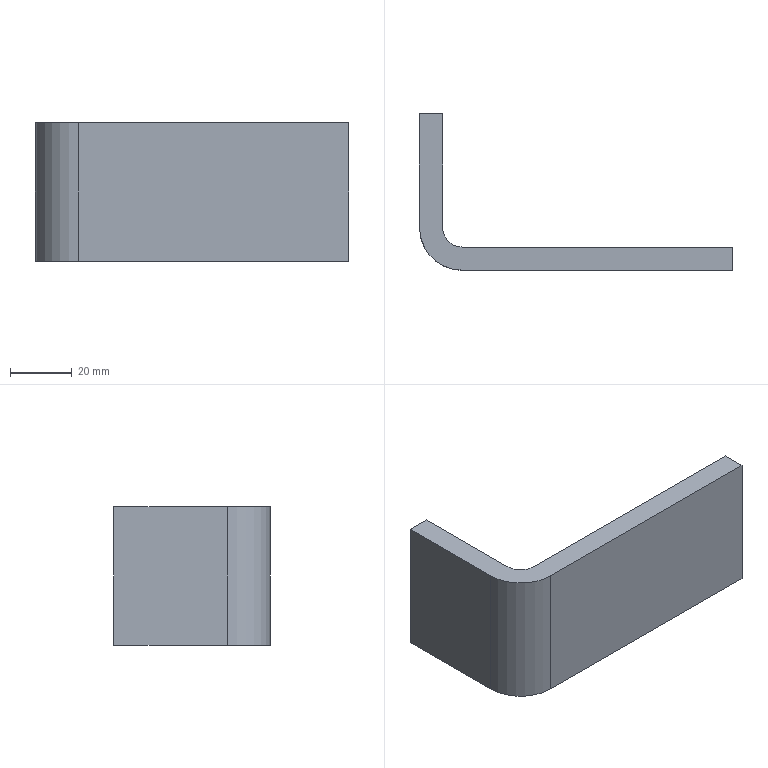Part | SolidWorks | features Extrusion 1 | 1 solid | 10 faces | box 101.6 x 50.8 x 45 mm | volume 47441 mm3 | plane 8 | cylinder 2 | commonest cylinder face diameters 12.7 x1 27.7 x1
STEP:
#1=CARTESIAN_POINT('',(-16.453,5.356,0.));
#2=VERTEX_POINT('',#1);
#3=CARTESIAN_POINT('',(-23.953,5.356,0.));
#4=VERTEX_POINT('',#3);
#5=CARTESIAN_POINT('',(-16.453,5.356,0.));
#6=DIRECTION('',(-1.,0.,0.));
#7=VECTOR('',#6,1000.);
#8=LINE('',#5,#7);
#9=EDGE_CURVE('',#2,#4,#8,.T.);
#10=ORIENTED_EDGE('',*,*,#9,.T.);
#11=CARTESIAN_POINT('',(-23.953,5.356,45.));
#12=VERTEX_POINT('',#11);
#13=CARTESIAN_POINT('',(-23.953,5.356,45.));
#14=DIRECTION('',(0.,0.,-1.));
#15=VECTOR('',#14,1000.);
#16=LINE('',#13,#15);
#17=EDGE_CURVE('',#12,#4,#16,.T.);
#18=ORIENTED_EDGE('',*,*,#17,.F.);
#19=CARTESIAN_POINT('',(-16.453,5.356,45.));
#20=VERTEX_POINT('',#19);
#21=CARTESIAN_POINT('',(-16.453,5.356,45.));
#22=DIRECTION('',(-1.,0.,0.));
#23=VECTOR('',#22,1000.);
#24=LINE('',#21,#23);
#25=EDGE_CURVE('',#20,#12,#24,.T.);
#26=ORIENTED_EDGE('',*,*,#25,.F.);
#27=CARTESIAN_POINT('',(-16.453,5.356,45.));
#28=DIRECTION('',(0.,0.,-1.));
#29=VECTOR('',#28,1000.);
#30=LINE('',#27,#29);
#31=EDGE_CURVE('',#20,#2,#30,.T.);
#32=ORIENTED_EDGE('',*,*,#31,.T.);
#33=EDGE_LOOP('',(#10,#18,#26,#32));
#34=FACE_OUTER_BOUND('',#33,.T.);
#35=CARTESIAN_POINT('',(-16.453,5.356,45.));
#36=DIRECTION('',(0.,-1.,0.));
#37=DIRECTION('',(1.,0.,0.));
#38=AXIS2_PLACEMENT_3D('',#35,#36,#37);
#39=PLANE('',#38);
#40=ADVANCED_FACE('',(#34),#39,.F.);
#41=CARTESIAN_POINT('',(-23.953,-31.594,0.));
#42=VERTEX_POINT('',#41);
#43=CARTESIAN_POINT('',(-23.953,5.356,0.));
#44=DIRECTION('',(0.,-1.,0.));
#45=VECTOR('',#44,1000.);
#46=LINE('',#43,#45);
#47=EDGE_CURVE('',#4,#42,#46,.T.);
#48=ORIENTED_EDGE('',*,*,#47,.T.);
#49=CARTESIAN_POINT('',(-23.953,-31.594,45.));
#50=VERTEX_POINT('',#49);
#51=CARTESIAN_POINT('',(-23.953,-31.594,45.));
#52=DIRECTION('',(0.,0.,-1.));
#53=VECTOR('',#52,1000.);
#54=LINE('',#51,#53);
#55=EDGE_CURVE('',#50,#42,#54,.T.);
#56=ORIENTED_EDGE('',*,*,#55,.F.);
#57=CARTESIAN_POINT('',(-23.953,5.356,45.));
#58=DIRECTION('',(0.,-1.,0.));
#59=VECTOR('',#58,1000.);
#60=LINE('',#57,#59);
#61=EDGE_CURVE('',#12,#50,#60,.T.);
#62=ORIENTED_EDGE('',*,*,#61,.F.);
#63=ORIENTED_EDGE('',*,*,#17,.T.);
#64=EDGE_LOOP('',(#48,#56,#62,#63));
#65=FACE_OUTER_BOUND('',#64,.T.);
#66=CARTESIAN_POINT('',(-23.953,5.356,45.));
#67=DIRECTION('',(1.,0.,0.));
#68=DIRECTION('',(0.,1.,0.));
#69=AXIS2_PLACEMENT_3D('',#66,#67,#68);
#70=PLANE('',#69);
#71=ADVANCED_FACE('',(#65),#70,.F.);
#72=CARTESIAN_POINT('',(-10.103,-45.444,0.));
#73=VERTEX_POINT('',#72);
#74=CARTESIAN_POINT('',(-10.103,-31.594,0.));
#75=DIRECTION('',(0.,0.,1.));
#76=DIRECTION('',(1.,0.,0.));
#77=AXIS2_PLACEMENT_3D('',#74,#75,#76);
#78=CIRCLE('',#77,13.85);
#79=EDGE_CURVE('',#42,#73,#78,.T.);
#80=ORIENTED_EDGE('',*,*,#79,.T.);
#81=CARTESIAN_POINT('',(-10.103,-45.444,45.));
#82=VERTEX_POINT('',#81);
#83=CARTESIAN_POINT('',(-10.103,-45.444,45.));
#84=DIRECTION('',(0.,0.,-1.));
#85=VECTOR('',#84,1000.);
#86=LINE('',#83,#85);
#87=EDGE_CURVE('',#82,#73,#86,.T.);
#88=ORIENTED_EDGE('',*,*,#87,.F.);
#89=CARTESIAN_POINT('',(-10.103,-31.594,45.));
#90=DIRECTION('',(0.,0.,1.));
#91=DIRECTION('',(1.,0.,0.));
#92=AXIS2_PLACEMENT_3D('',#89,#90,#91);
#93=CIRCLE('',#92,13.85);
#94=EDGE_CURVE('',#50,#82,#93,.T.);
#95=ORIENTED_EDGE('',*,*,#94,.F.);
#96=ORIENTED_EDGE('',*,*,#55,.T.);
#97=EDGE_LOOP('',(#80,#88,#95,#96));
#98=FACE_OUTER_BOUND('',#97,.T.);
#99=CARTESIAN_POINT('',(-10.103,-31.594,45.));
#100=DIRECTION('',(0.,0.,-1.));
#101=DIRECTION('',(-1.,0.,0.));
#102=AXIS2_PLACEMENT_3D('',#99,#100,#101);
#103=CYLINDRICAL_SURFACE('',#102,13.85);
#104=ADVANCED_FACE('',(#98),#103,.T.);
#105=CARTESIAN_POINT('',(77.647,-45.444,0.));
#106=VERTEX_POINT('',#105);
#107=CARTESIAN_POINT('',(-10.103,-45.444,0.));
#108=DIRECTION('',(1.,0.,0.));
#109=VECTOR('',#108,1000.);
#110=LINE('',#107,#109);
#111=EDGE_CURVE('',#73,#106,#110,.T.);
#112=ORIENTED_EDGE('',*,*,#111,.T.);
#113=CARTESIAN_POINT('',(77.647,-45.444,45.));
#114=VERTEX_POINT('',#113);
#115=CARTESIAN_POINT('',(77.647,-45.444,45.));
#116=DIRECTION('',(0.,0.,-1.));
#117=VECTOR('',#116,1000.);
#118=LINE('',#115,#117);
#119=EDGE_CURVE('',#114,#106,#118,.T.);
#120=ORIENTED_EDGE('',*,*,#119,.F.);
#121=CARTESIAN_POINT('',(-10.103,-45.444,45.));
#122=DIRECTION('',(1.,0.,0.));
#123=VECTOR('',#122,1000.);
#124=LINE('',#121,#123);
#125=EDGE_CURVE('',#82,#114,#124,.T.);
#126=ORIENTED_EDGE('',*,*,#125,.F.);
#127=ORIENTED_EDGE('',*,*,#87,.T.);
#128=EDGE_LOOP('',(#112,#120,#126,#127));
#129=FACE_OUTER_BOUND('',#128,.T.);
#130=CARTESIAN_POINT('',(-10.103,-45.444,45.));
#131=DIRECTION('',(0.,1.,0.));
#132=DIRECTION('',(0.,0.,1.));
#133=AXIS2_PLACEMENT_3D('',#130,#131,#132);
#134=PLANE('',#133);
#135=ADVANCED_FACE('',(#129),#134,.F.);
#136=CARTESIAN_POINT('',(77.647,-37.944,0.));
#137=VERTEX_POINT('',#136);
#138=CARTESIAN_POINT('',(77.647,-45.444,0.));
#139=DIRECTION('',(0.,1.,0.));
#140=VECTOR('',#139,1000.);
#141=LINE('',#138,#140);
#142=EDGE_CURVE('',#106,#137,#141,.T.);
#143=ORIENTED_EDGE('',*,*,#142,.T.);
#144=CARTESIAN_POINT('',(77.647,-37.944,45.));
#145=VERTEX_POINT('',#144);
#146=CARTESIAN_POINT('',(77.647,-37.944,45.));
#147=DIRECTION('',(0.,0.,-1.));
#148=VECTOR('',#147,1000.);
#149=LINE('',#146,#148);
#150=EDGE_CURVE('',#145,#137,#149,.T.);
#151=ORIENTED_EDGE('',*,*,#150,.F.);
#152=CARTESIAN_POINT('',(77.647,-45.444,45.));
#153=DIRECTION('',(0.,1.,0.));
#154=VECTOR('',#153,1000.);
#155=LINE('',#152,#154);
#156=EDGE_CURVE('',#114,#145,#155,.T.);
#157=ORIENTED_EDGE('',*,*,#156,.F.);
#158=ORIENTED_EDGE('',*,*,#119,.T.);
#159=EDGE_LOOP('',(#143,#151,#157,#158));
#160=FACE_OUTER_BOUND('',#159,.T.);
#161=CARTESIAN_POINT('',(77.647,-45.444,45.));
#162=DIRECTION('',(-1.,0.,0.));
#163=DIRECTION('',(0.,0.,1.));
#164=AXIS2_PLACEMENT_3D('',#161,#162,#163);
#165=PLANE('',#164);
#166=ADVANCED_FACE('',(#160),#165,.F.);
#167=CARTESIAN_POINT('',(-10.103,-37.944,0.));
#168=VERTEX_POINT('',#167);
#169=CARTESIAN_POINT('',(77.647,-37.944,0.));
#170=DIRECTION('',(-1.,0.,0.));
#171=VECTOR('',#170,1000.);
#172=LINE('',#169,#171);
#173=EDGE_CURVE('',#137,#168,#172,.T.);
#174=ORIENTED_EDGE('',*,*,#173,.T.);
#175=CARTESIAN_POINT('',(-10.103,-37.944,45.));
#176=VERTEX_POINT('',#175);
#177=CARTESIAN_POINT('',(-10.103,-37.944,45.));
#178=DIRECTION('',(0.,0.,-1.));
#179=VECTOR('',#178,1000.);
#180=LINE('',#177,#179);
#181=EDGE_CURVE('',#176,#168,#180,.T.);
#182=ORIENTED_EDGE('',*,*,#181,.F.);
#183=CARTESIAN_POINT('',(77.647,-37.944,45.));
#184=DIRECTION('',(-1.,0.,0.));
#185=VECTOR('',#184,1000.);
#186=LINE('',#183,#185);
#187=EDGE_CURVE('',#145,#176,#186,.T.);
#188=ORIENTED_EDGE('',*,*,#187,.F.);
#189=ORIENTED_EDGE('',*,*,#150,.T.);
#190=EDGE_LOOP('',(#174,#182,#188,#189));
#191=FACE_OUTER_BOUND('',#190,.T.);
#192=CARTESIAN_POINT('',(77.647,-37.944,45.));
#193=DIRECTION('',(0.,-1.,0.));
#194=DIRECTION('',(1.,0.,0.));
#195=AXIS2_PLACEMENT_3D('',#192,#193,#194);
#196=PLANE('',#195);
#197=ADVANCED_FACE('',(#191),#196,.F.);
#198=CARTESIAN_POINT('',(-16.453,-31.594,0.));
#199=VERTEX_POINT('',#198);
#200=CARTESIAN_POINT('',(-10.103,-31.594,0.));
#201=DIRECTION('',(0.,0.,-1.));
#202=DIRECTION('',(-1.,0.,0.));
#203=AXIS2_PLACEMENT_3D('',#200,#201,#202);
#204=CIRCLE('',#203,6.35);
#205=EDGE_CURVE('',#168,#199,#204,.T.);
#206=ORIENTED_EDGE('',*,*,#205,.T.);
#207=CARTESIAN_POINT('',(-16.453,-31.594,45.));
#208=VERTEX_POINT('',#207);
#209=CARTESIAN_POINT('',(-16.453,-31.594,45.));
#210=DIRECTION('',(0.,0.,-1.));
#211=VECTOR('',#210,1000.);
#212=LINE('',#209,#211);
#213=EDGE_CURVE('',#208,#199,#212,.T.);
#214=ORIENTED_EDGE('',*,*,#213,.F.);
#215=CARTESIAN_POINT('',(-10.103,-31.594,45.));
#216=DIRECTION('',(0.,0.,-1.));
#217=DIRECTION('',(-1.,0.,0.));
#218=AXIS2_PLACEMENT_3D('',#215,#216,#217);
#219=CIRCLE('',#218,6.35);
#220=EDGE_CURVE('',#176,#208,#219,.T.);
#221=ORIENTED_EDGE('',*,*,#220,.F.);
#222=ORIENTED_EDGE('',*,*,#181,.T.);
#223=EDGE_LOOP('',(#206,#214,#221,#222));
#224=FACE_OUTER_BOUND('',#223,.T.);
#225=CARTESIAN_POINT('',(-10.103,-31.594,45.));
#226=DIRECTION('',(0.,0.,-1.));
#227=DIRECTION('',(-1.,0.,0.));
#228=AXIS2_PLACEMENT_3D('',#225,#226,#227);
#229=CYLINDRICAL_SURFACE('',#228,6.35);
#230=ADVANCED_FACE('',(#224),#229,.F.);
#231=CARTESIAN_POINT('',(-16.453,-31.594,0.));
#232=DIRECTION('',(0.,1.,0.));
#233=VECTOR('',#232,1000.);
#234=LINE('',#231,#233);
#235=EDGE_CURVE('',#199,#2,#234,.T.);
#236=ORIENTED_EDGE('',*,*,#235,.T.);
#237=ORIENTED_EDGE('',*,*,#31,.F.);
#238=CARTESIAN_POINT('',(-16.453,-31.594,45.));
#239=DIRECTION('',(0.,1.,0.));
#240=VECTOR('',#239,1000.);
#241=LINE('',#238,#240);
#242=EDGE_CURVE('',#208,#20,#241,.T.);
#243=ORIENTED_EDGE('',*,*,#242,.F.);
#244=ORIENTED_EDGE('',*,*,#213,.T.);
#245=EDGE_LOOP('',(#236,#237,#243,#244));
#246=FACE_OUTER_BOUND('',#245,.T.);
#247=CARTESIAN_POINT('',(-16.453,-31.594,45.));
#248=DIRECTION('',(-1.,0.,0.));
#249=DIRECTION('',(0.,-1.,0.));
#250=AXIS2_PLACEMENT_3D('',#247,#248,#249);
#251=PLANE('',#250);
#252=ADVANCED_FACE('',(#246),#251,.F.);
#253=ORIENTED_EDGE('',*,*,#25,.T.);
#254=ORIENTED_EDGE('',*,*,#61,.T.);
#255=ORIENTED_EDGE('',*,*,#94,.T.);
#256=ORIENTED_EDGE('',*,*,#125,.T.);
#257=ORIENTED_EDGE('',*,*,#156,.T.);
#258=ORIENTED_EDGE('',*,*,#187,.T.);
#259=ORIENTED_EDGE('',*,*,#220,.T.);
#260=ORIENTED_EDGE('',*,*,#242,.T.);
#261=EDGE_LOOP('',(#253,#254,#255,#256,#257,#258,#259,#260));
#262=FACE_OUTER_BOUND('',#261,.T.);
#263=CARTESIAN_POINT('',(-10.103,-31.594,45.));
#264=DIRECTION('',(0.,0.,1.));
#265=DIRECTION('',(1.,0.,0.));
#266=AXIS2_PLACEMENT_3D('',#263,#264,#265);
#267=PLANE('',#266);
#268=ADVANCED_FACE('',(#262),#267,.T.);
#269=ORIENTED_EDGE('',*,*,#9,.F.);
#270=ORIENTED_EDGE('',*,*,#235,.F.);
#271=ORIENTED_EDGE('',*,*,#205,.F.);
#272=ORIENTED_EDGE('',*,*,#173,.F.);
#273=ORIENTED_EDGE('',*,*,#142,.F.);
#274=ORIENTED_EDGE('',*,*,#111,.F.);
#275=ORIENTED_EDGE('',*,*,#79,.F.);
#276=ORIENTED_EDGE('',*,*,#47,.F.);
#277=EDGE_LOOP('',(#269,#270,#271,#272,#273,#274,#275,#276));
#278=FACE_OUTER_BOUND('',#277,.T.);
#279=CARTESIAN_POINT('',(-10.103,-31.594,0.));
#280=DIRECTION('',(0.,0.,1.));
#281=DIRECTION('',(1.,0.,0.));
#282=AXIS2_PLACEMENT_3D('',#279,#280,#281);
#283=PLANE('',#282);
#284=ADVANCED_FACE('',(#278),#283,.F.);
#285=CLOSED_SHELL('',(#40,#71,#104,#135,#166,#197,#230,#252,#268,#284));
#286=MANIFOLD_SOLID_BREP('',#285);
#287=CARTESIAN_POINT('',(0.,0.,0.));
#288=DIRECTION('',(0.,0.,1.));
#289=DIRECTION('',(1.,0.,0.));
#290=AXIS2_PLACEMENT_3D('',#287,#288,#289);
#291=(LENGTH_UNIT()NAMED_UNIT(*)SI_UNIT(.MILLI.,.METRE.));
#292=UNCERTAINTY_MEASURE_WITH_UNIT(LENGTH_MEASURE(0.00001),#291,'','');
#293=(NAMED_UNIT(*)PLANE_ANGLE_UNIT()SI_UNIT($,.RADIAN.));
#294=(NAMED_UNIT(*)SI_UNIT($,.STERADIAN.)SOLID_ANGLE_UNIT());
#295=(GEOMETRIC_REPRESENTATION_CONTEXT(3)GLOBAL_UNCERTAINTY_ASSIGNED_CONTEXT((#292))GLOBAL_UNIT_ASSIGNED_CONTEXT((#291,#293,#294))REPRESENTATION_CONTEXT('',''));
#296=ADVANCED_BREP_SHAPE_REPRESENTATION('',(#286,#290),#295);